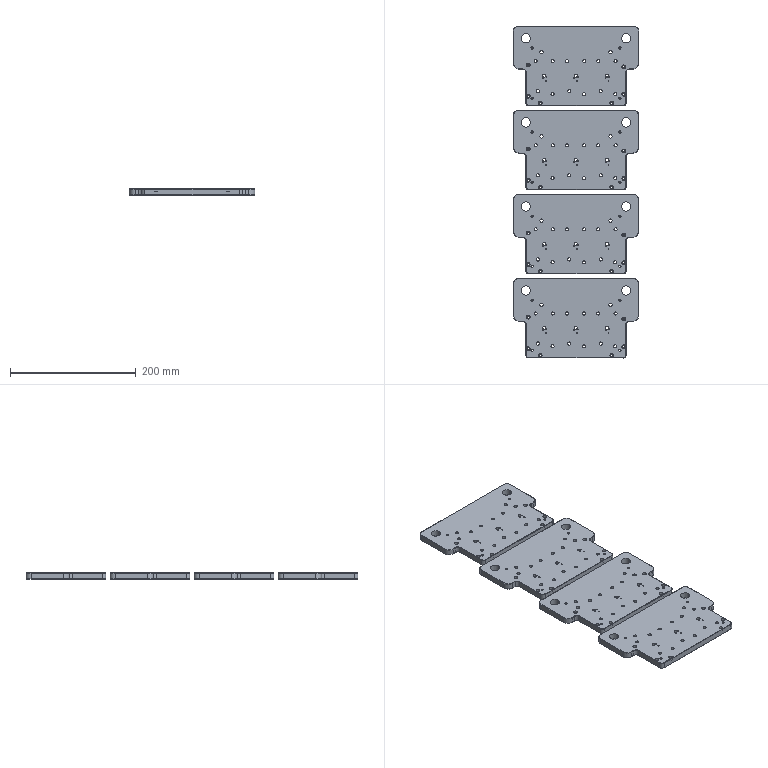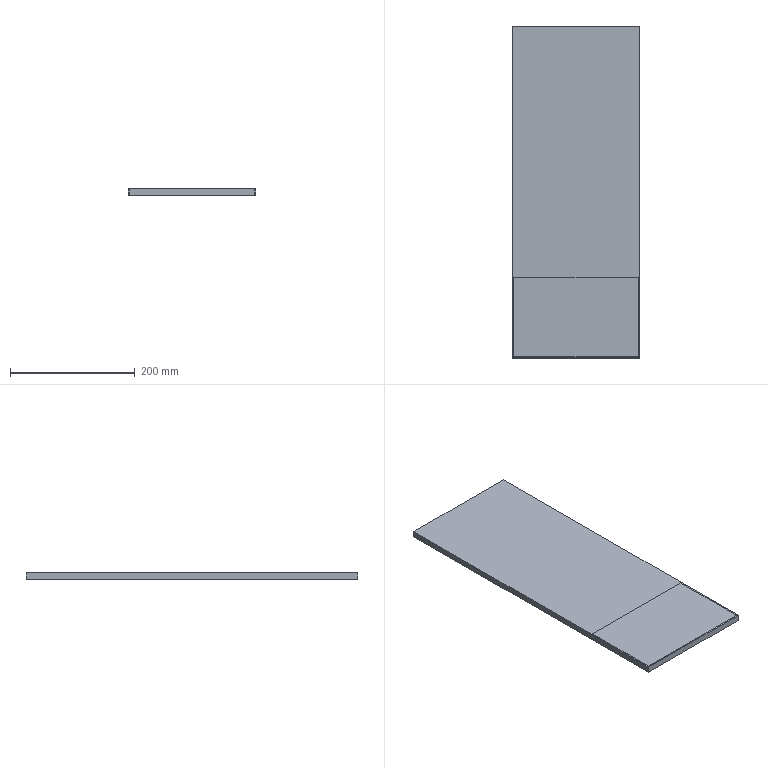CAM job | NX | 3-axis milling, drilling | part box 200 x 529 x 10 mm | stock box 204 x 533 x 10 mm
Tools:
number,name,description,diameter,corner_radius,flute_length,length,flutes
6,D6,Milling Tool-5 Parameters,6.0,0.0,50.0,75.0,2
2,D4A45,Milling Tool-5 Parameters,4.0,0.0,2.0,2.0,2
4,D4,Milling Tool-5 Parameters,4.0,0.0,50.0,75.0,2
17,1.7ZT,Drilling Tool,1.7,0.0,35.0,50.0,2
19,0.97ZT,Drilling Tool,0.97,0.0,35.0,50.0,2
15,3.5ZT,Drilling Tool,3.5,0.0,35.0,50.0,2
3,D3,Milling Tool-5 Parameters,3.0,0.0,50.0,75.0,2
Operations:
program,operation,operation_type,tool,method,geometry_group,spindle_rpm,surface_speed,feed_per_tooth,feed_cut,feed_plunge,cut_length_mm,path_length_mm,cut_time_min,machine_time_min
1吸,ZLEVEL_PROFILE_1_COPY_1_COPY,ZLevelMilling,D4A45,METHOD,A,9500.0,179.0,0.0526,1000.0,100.0,4416.129,23551.823,4.416,6.33
1吸,HOLE_MILLING,CylinderMilling,D4,METHOD,A,9500.0,179.0,0.1158,2200.0,100.0,1926.089,4583.624,0.8755,1.141
1吸,ZLEVEL_PROFILE_COPY_COPY_1_COPY,ZLevelMilling,D6,METHOD,A,9500.0,179.0,0.1158,2200.0,1000.0,52224.405,52938.834,23.821,23.893
1吸,ZLEVEL_PROFILE_COPY_COPY_COPY_COPY,ZLevelMilling,D6,MILL_FINISH,A,9500.0,119.0,0.0632,1200.0,1000.0,2614.98,3591.816,2.181,2.279
2,DRILLING_COPY,Operation,D4A45,METHOD,B,5000.0,62.0,0.025,250.0,0.0,147.6,1131.306,0.5904,0.6888
2,DRILLING_COPY_COPY_COPY_COPY_COPY_COPY,Operation,1.7ZT,METHOD,B,2000.0,10.0,0.03,120.0,0.0,45.032,256.244,0.3753,0.3964
2,DRILLING_COPY_COPY_COPY_COPY_COPY_COPY_COPY,Operation,0.97ZT,METHOD,B,2000.0,6.0,0.025,100.0,0.0,133.123,478.218,1.331,1.366
2,DRILLING_COPY_COPY_COPY_COPY_COPY,Operation,3.5ZT,METHOD,B,1910.0,21.0,0.0471,180.0,0.0,69.309,467.799,0.3851,0.4249
2,DRILLING_COPY_COPY_COPY_COPY_COPY_COPY_1,Operation,3.5ZT,METHOD,B,1910.0,21.0,0.0471,180.0,0.0,62.206,493.557,0.3456,0.3887
2,DRILLING_COPY_COPY_COPY_COPY_COPY_COPY_1_COPY,Operation,3.5ZT,METHOD,B,1910.0,21.0,0.0471,180.0,0.0,264.376,1024.27,1.469,1.545
2,HOLE_MILLING_COPY,CylinderMilling,D4,METHOD,B,9500.0,179.0,0.1158,2200.0,100.0,498.56,1203.191,0.2266,0.2971
2,HOLE_MILLING_1,CylinderMilling,D6,METHOD,B,9500.0,179.0,0.1158,2200.0,100.0,1866.676,2186.676,0.8485,0.8805
2,HOLE_MILLING_COPY_COPY,CylinderMilling,D3,METHOD,B,9500.0,89.0,0.0526,1000.0,100.0,3100.214,4501.638,3.1,3.24
2,HOLE_MILLING_COPY_COPY_COPY,CylinderMilling,D3,METHOD,B,9500.0,89.0,0.0526,1000.0,100.0,337.858,590.858,0.3379,0.3632
2,ZLEVEL_PROFILE_1_COPY_1_COPY_COPY,ZLevelMilling,D4A45,METHOD,B,9500.0,179.0,0.0526,1000.0,100.0,1098.108,5617.597,1.098,1.55
2,刀补6,CylinderMilling,D6,METHOD,B,9500.0,179.0,0.0632,1200.0,100.0,377.128,676.128,0.3143,0.3442
2,刀补,CylinderMilling,D3,METHOD,B,9500.0,89.0,0.0526,1000.0,100.0,87.7,340.7,0.0877,0.113
2,刀补_COPY,CylinderMilling,D3,METHOD,B,9500.0,89.0,0.0526,1000.0,100.0,780.846,2235.334,0.7808,0.9263